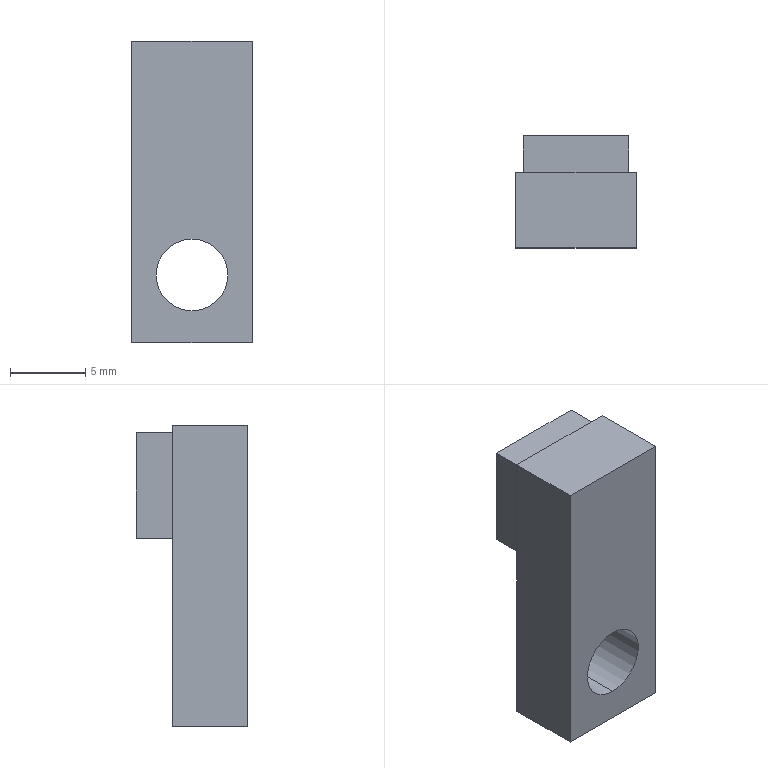Part | STEP file | 1_id1454_x_t | 1 solid | 13 faces | box 8 x 7.4 x 20 mm | volume 828.53 mm3 | plane 11 | cylinder 2 | commonest cylinder face diameters 4.763 x2
STEP:
#1=CARTESIAN_POINT('',(0.,0.,0.));
#2=DIRECTION('',(0.,0.,1.));
#3=DIRECTION('',(1.,0.,0.));
#4=AXIS2_PLACEMENT_3D('',#1,#2,#3);
#5=CARTESIAN_POINT('',(973.367,32.427,9.687));
#6=VERTEX_POINT('',#5);
#7=CARTESIAN_POINT('',(965.367,32.427,9.687));
#8=VERTEX_POINT('',#7);
#9=CARTESIAN_POINT('',(973.367,32.427,9.687));
#10=DIRECTION('',(-1.,0.,0.));
#11=VECTOR('',#10,1.);
#12=LINE('',#9,#11);
#13=CARTESIAN_POINT('',(969.367,32.427,9.687));
#14=DIRECTION('',(0.,1.,0.));
#15=DIRECTION('',(1.,0.,0.));
#16=AXIS2_PLACEMENT_3D('',#13,#14,#15);
#17=PLANE('',#16);
#18=CARTESIAN_POINT('',(4.,0.));
#19=DIRECTION('',(-1.,0.));
#20=VECTOR('',#19,1.);
#21=LINE('',#18,#20);
#22=(GEOMETRIC_REPRESENTATION_CONTEXT(2)PARAMETRIC_REPRESENTATION_CONTEXT()REPRESENTATION_CONTEXT('',''));
#23=DEFINITIONAL_REPRESENTATION('',(#21),#22);
#24=PCURVE('',#17,#23);
#25=CARTESIAN_POINT('',(969.367,29.927,9.687));
#26=DIRECTION('',(0.,0.,-1.));
#27=DIRECTION('',(0.,1.,0.));
#28=AXIS2_PLACEMENT_3D('',#25,#26,#27);
#29=PLANE('',#28);
#30=CARTESIAN_POINT('',(2.5,4.));
#31=DIRECTION('',(0.,-1.));
#32=VECTOR('',#31,1.);
#33=LINE('',#30,#32);
#34=(GEOMETRIC_REPRESENTATION_CONTEXT(2)PARAMETRIC_REPRESENTATION_CONTEXT()REPRESENTATION_CONTEXT('',''));
#35=DEFINITIONAL_REPRESENTATION('',(#33),#34);
#36=PCURVE('',#29,#35);
#37=SURFACE_CURVE('',#12,(#24,#36),.PCURVE_S1.);
#38=EDGE_CURVE('',#6,#8,#37,.T.);
#39=ORIENTED_EDGE('',*,*,#38,.T.);
#40=CARTESIAN_POINT('',(965.367,32.427,29.687));
#41=VERTEX_POINT('',#40);
#42=CARTESIAN_POINT('',(965.367,32.427,29.687));
#43=DIRECTION('',(0.,0.,-1.));
#44=VECTOR('',#43,1.);
#45=LINE('',#42,#44);
#46=CARTESIAN_POINT('',(-4.,-20.));
#47=DIRECTION('',(0.,1.));
#48=VECTOR('',#47,1.);
#49=LINE('',#46,#48);
#50=(GEOMETRIC_REPRESENTATION_CONTEXT(2)PARAMETRIC_REPRESENTATION_CONTEXT()REPRESENTATION_CONTEXT('',''));
#51=DEFINITIONAL_REPRESENTATION('',(#49),#50);
#52=PCURVE('',#17,#51);
#53=CARTESIAN_POINT('',(965.367,29.927,9.687));
#54=DIRECTION('',(-1.,0.,0.));
#55=DIRECTION('',(0.,-1.,0.));
#56=AXIS2_PLACEMENT_3D('',#53,#54,#55);
#57=PLANE('',#56);
#58=CARTESIAN_POINT('',(-2.5,20.));
#59=DIRECTION('',(0.,-1.));
#60=VECTOR('',#59,1.);
#61=LINE('',#58,#60);
#62=(GEOMETRIC_REPRESENTATION_CONTEXT(2)PARAMETRIC_REPRESENTATION_CONTEXT()REPRESENTATION_CONTEXT('',''));
#63=DEFINITIONAL_REPRESENTATION('',(#61),#62);
#64=PCURVE('',#57,#63);
#65=SURFACE_CURVE('',#45,(#52,#64),.PCURVE_S1.);
#66=EDGE_CURVE('',#41,#8,#65,.T.);
#67=ORIENTED_EDGE('',*,*,#66,.F.);
#68=CARTESIAN_POINT('',(973.367,32.427,29.687));
#69=VERTEX_POINT('',#68);
#70=CARTESIAN_POINT('',(965.367,32.427,29.687));
#71=DIRECTION('',(1.,0.,0.));
#72=VECTOR('',#71,1.);
#73=LINE('',#70,#72);
#74=CARTESIAN_POINT('',(-4.,-20.));
#75=DIRECTION('',(1.,0.));
#76=VECTOR('',#75,1.);
#77=LINE('',#74,#76);
#78=(GEOMETRIC_REPRESENTATION_CONTEXT(2)PARAMETRIC_REPRESENTATION_CONTEXT()REPRESENTATION_CONTEXT('',''));
#79=DEFINITIONAL_REPRESENTATION('',(#77),#78);
#80=PCURVE('',#17,#79);
#81=CARTESIAN_POINT('',(969.367,29.927,29.687));
#82=DIRECTION('',(0.,0.,1.));
#83=DIRECTION('',(1.,0.,0.));
#84=AXIS2_PLACEMENT_3D('',#81,#82,#83);
#85=PLANE('',#84);
#86=CARTESIAN_POINT('',(-4.,2.5));
#87=DIRECTION('',(1.,0.));
#88=VECTOR('',#87,1.);
#89=LINE('',#86,#88);
#90=(GEOMETRIC_REPRESENTATION_CONTEXT(2)PARAMETRIC_REPRESENTATION_CONTEXT()REPRESENTATION_CONTEXT('',''));
#91=DEFINITIONAL_REPRESENTATION('',(#89),#90);
#92=PCURVE('',#85,#91);
#93=SURFACE_CURVE('',#73,(#80,#92),.PCURVE_S1.);
#94=EDGE_CURVE('',#41,#69,#93,.T.);
#95=ORIENTED_EDGE('',*,*,#94,.T.);
#96=CARTESIAN_POINT('',(973.367,32.427,29.687));
#97=DIRECTION('',(0.,0.,-1.));
#98=VECTOR('',#97,1.);
#99=LINE('',#96,#98);
#100=CARTESIAN_POINT('',(4.,-20.));
#101=DIRECTION('',(0.,1.));
#102=VECTOR('',#101,1.);
#103=LINE('',#100,#102);
#104=(GEOMETRIC_REPRESENTATION_CONTEXT(2)PARAMETRIC_REPRESENTATION_CONTEXT()REPRESENTATION_CONTEXT('',''));
#105=DEFINITIONAL_REPRESENTATION('',(#103),#104);
#106=PCURVE('',#17,#105);
#107=CARTESIAN_POINT('',(973.367,29.927,9.687));
#108=DIRECTION('',(1.,0.,0.));
#109=DIRECTION('',(0.,-1.,0.));
#110=AXIS2_PLACEMENT_3D('',#107,#108,#109);
#111=PLANE('',#110);
#112=CARTESIAN_POINT('',(-2.5,-20.));
#113=DIRECTION('',(0.,1.));
#114=VECTOR('',#113,1.);
#115=LINE('',#112,#114);
#116=(GEOMETRIC_REPRESENTATION_CONTEXT(2)PARAMETRIC_REPRESENTATION_CONTEXT()REPRESENTATION_CONTEXT('',''));
#117=DEFINITIONAL_REPRESENTATION('',(#115),#116);
#118=PCURVE('',#111,#117);
#119=SURFACE_CURVE('',#99,(#106,#118),.PCURVE_S1.);
#120=EDGE_CURVE('',#69,#6,#119,.T.);
#121=ORIENTED_EDGE('',*,*,#120,.T.);
#122=EDGE_LOOP('',(#39,#67,#95,#121));
#123=FACE_BOUND('',#122,.T.);
#124=CARTESIAN_POINT('',(969.367,32.427,16.569));
#125=VERTEX_POINT('',#124);
#126=CARTESIAN_POINT('',(969.367,32.427,11.806));
#127=VERTEX_POINT('',#126);
#128=CARTESIAN_POINT('',(969.367,32.427,14.187));
#129=DIRECTION('',(0.,-1.,0.));
#130=DIRECTION('',(0.,0.,1.));
#131=AXIS2_PLACEMENT_3D('',#128,#129,#130);
#132=CIRCLE('',#131,2.381);
#133=CARTESIAN_POINT('',(0.,-6.881));
#134=CARTESIAN_POINT('',(-4.124,-6.881));
#135=CARTESIAN_POINT('',(-2.062,-3.309));
#136=CARTESIAN_POINT('',(0.,0.2625));
#137=CARTESIAN_POINT('',(2.062,-3.309));
#138=CARTESIAN_POINT('',(4.124,-6.881));
#139=CARTESIAN_POINT('',(0.,-6.881));
#140=(BOUNDED_CURVE()B_SPLINE_CURVE(2,(#133,#134,#135,#136,#137,#138,#139),.UNSPECIFIED.,.T.,.F.)B_SPLINE_CURVE_WITH_KNOTS((1,2,2,2,2,1),(-2.094,0.,2.094,4.189,6.283,8.378),.UNSPECIFIED.)CURVE()GEOMETRIC_REPRESENTATION_ITEM()RATIONAL_B_SPLINE_CURVE((1.,0.5,1.,0.5,1.,0.5,1.))REPRESENTATION_ITEM(''));
#141=(GEOMETRIC_REPRESENTATION_CONTEXT(2)PARAMETRIC_REPRESENTATION_CONTEXT()REPRESENTATION_CONTEXT('',''));
#142=DEFINITIONAL_REPRESENTATION('',(#140),#141);
#143=PCURVE('',#17,#142);
#144=CARTESIAN_POINT('',(969.367,32.427,14.187));
#145=DIRECTION('',(0.,1.,0.));
#146=DIRECTION('',(0.,0.,1.));
#147=AXIS2_PLACEMENT_3D('',#144,#145,#146);
#148=CYLINDRICAL_SURFACE('',#147,2.381);
#149=CARTESIAN_POINT('',(6.283,0.));
#150=DIRECTION('',(-1.,0.));
#151=VECTOR('',#150,1.);
#152=LINE('',#149,#151);
#153=(GEOMETRIC_REPRESENTATION_CONTEXT(2)PARAMETRIC_REPRESENTATION_CONTEXT()REPRESENTATION_CONTEXT('',''));
#154=DEFINITIONAL_REPRESENTATION('',(#152),#153);
#155=PCURVE('',#148,#154);
#156=SURFACE_CURVE('',#132,(#143,#155),.PCURVE_S1.);
#157=EDGE_CURVE('',#125,#127,#156,.T.);
#158=ORIENTED_EDGE('',*,*,#157,.T.);
#159=CARTESIAN_POINT('',(969.367,32.427,14.187));
#160=DIRECTION('',(0.,-1.,0.));
#161=DIRECTION('',(0.,0.,-1.));
#162=AXIS2_PLACEMENT_3D('',#159,#160,#161);
#163=CIRCLE('',#162,2.381);
#164=CARTESIAN_POINT('',(0.,-2.119));
#165=CARTESIAN_POINT('',(4.124,-2.119));
#166=CARTESIAN_POINT('',(2.062,-5.691));
#167=CARTESIAN_POINT('',(0.,-9.262));
#168=CARTESIAN_POINT('',(-2.062,-5.691));
#169=CARTESIAN_POINT('',(-4.124,-2.119));
#170=CARTESIAN_POINT('',(0.,-2.119));
#171=(BOUNDED_CURVE()B_SPLINE_CURVE(2,(#164,#165,#166,#167,#168,#169,#170),.UNSPECIFIED.,.T.,.F.)B_SPLINE_CURVE_WITH_KNOTS((1,2,2,2,2,1),(-2.094,0.,2.094,4.189,6.283,8.378),.UNSPECIFIED.)CURVE()GEOMETRIC_REPRESENTATION_ITEM()RATIONAL_B_SPLINE_CURVE((1.,0.5,1.,0.5,1.,0.5,1.))REPRESENTATION_ITEM(''));
#172=(GEOMETRIC_REPRESENTATION_CONTEXT(2)PARAMETRIC_REPRESENTATION_CONTEXT()REPRESENTATION_CONTEXT('',''));
#173=DEFINITIONAL_REPRESENTATION('',(#171),#172);
#174=PCURVE('',#17,#173);
#175=CARTESIAN_POINT('',(969.367,32.427,14.187));
#176=DIRECTION('',(0.,1.,0.));
#177=DIRECTION('',(0.,0.,1.));
#178=AXIS2_PLACEMENT_3D('',#175,#176,#177);
#179=CYLINDRICAL_SURFACE('',#178,2.381);
#180=CARTESIAN_POINT('',(3.142,0.));
#181=DIRECTION('',(-1.,0.));
#182=VECTOR('',#181,1.);
#183=LINE('',#180,#182);
#184=(GEOMETRIC_REPRESENTATION_CONTEXT(2)PARAMETRIC_REPRESENTATION_CONTEXT()REPRESENTATION_CONTEXT('',''));
#185=DEFINITIONAL_REPRESENTATION('',(#183),#184);
#186=PCURVE('',#179,#185);
#187=SURFACE_CURVE('',#163,(#174,#186),.PCURVE_S1.);
#188=EDGE_CURVE('',#127,#125,#187,.T.);
#189=ORIENTED_EDGE('',*,*,#188,.T.);
#190=EDGE_LOOP('',(#158,#189));
#191=FACE_BOUND('',#190,.T.);
#192=CARTESIAN_POINT('',(972.867,32.427,22.187));
#193=VERTEX_POINT('',#192);
#194=CARTESIAN_POINT('',(965.867,32.427,22.187));
#195=VERTEX_POINT('',#194);
#196=CARTESIAN_POINT('',(972.867,32.427,22.187));
#197=DIRECTION('',(-1.,0.,0.));
#198=VECTOR('',#197,1.);
#199=LINE('',#196,#198);
#200=CARTESIAN_POINT('',(3.5,-12.5));
#201=DIRECTION('',(-1.,0.));
#202=VECTOR('',#201,1.);
#203=LINE('',#200,#202);
#204=(GEOMETRIC_REPRESENTATION_CONTEXT(2)PARAMETRIC_REPRESENTATION_CONTEXT()REPRESENTATION_CONTEXT('',''));
#205=DEFINITIONAL_REPRESENTATION('',(#203),#204);
#206=PCURVE('',#17,#205);
#207=CARTESIAN_POINT('',(972.867,32.427,22.187));
#208=DIRECTION('',(0.,0.,-1.));
#209=DIRECTION('',(0.,1.,0.));
#210=AXIS2_PLACEMENT_3D('',#207,#208,#209);
#211=PLANE('',#210);
#212=CARTESIAN_POINT('',(0.,0.));
#213=DIRECTION('',(0.,-1.));
#214=VECTOR('',#213,1.);
#215=LINE('',#212,#214);
#216=(GEOMETRIC_REPRESENTATION_CONTEXT(2)PARAMETRIC_REPRESENTATION_CONTEXT()REPRESENTATION_CONTEXT('',''));
#217=DEFINITIONAL_REPRESENTATION('',(#215),#216);
#218=PCURVE('',#211,#217);
#219=SURFACE_CURVE('',#199,(#206,#218),.PCURVE_S1.);
#220=EDGE_CURVE('',#193,#195,#219,.T.);
#221=ORIENTED_EDGE('',*,*,#220,.F.);
#222=CARTESIAN_POINT('',(972.867,32.427,29.187));
#223=VERTEX_POINT('',#222);
#224=CARTESIAN_POINT('',(972.867,32.427,29.187));
#225=DIRECTION('',(0.,0.,-1.));
#226=VECTOR('',#225,1.);
#227=LINE('',#224,#226);
#228=CARTESIAN_POINT('',(3.5,-19.5));
#229=DIRECTION('',(0.,1.));
#230=VECTOR('',#229,1.);
#231=LINE('',#228,#230);
#232=(GEOMETRIC_REPRESENTATION_CONTEXT(2)PARAMETRIC_REPRESENTATION_CONTEXT()REPRESENTATION_CONTEXT('',''));
#233=DEFINITIONAL_REPRESENTATION('',(#231),#232);
#234=PCURVE('',#17,#233);
#235=CARTESIAN_POINT('',(972.867,32.427,29.187));
#236=DIRECTION('',(1.,0.,0.));
#237=DIRECTION('',(0.,-1.,0.));
#238=AXIS2_PLACEMENT_3D('',#235,#236,#237);
#239=PLANE('',#238);
#240=CARTESIAN_POINT('',(0.,0.));
#241=DIRECTION('',(0.,1.));
#242=VECTOR('',#241,1.);
#243=LINE('',#240,#242);
#244=(GEOMETRIC_REPRESENTATION_CONTEXT(2)PARAMETRIC_REPRESENTATION_CONTEXT()REPRESENTATION_CONTEXT('',''));
#245=DEFINITIONAL_REPRESENTATION('',(#243),#244);
#246=PCURVE('',#239,#245);
#247=SURFACE_CURVE('',#227,(#234,#246),.PCURVE_S1.);
#248=EDGE_CURVE('',#223,#193,#247,.T.);
#249=ORIENTED_EDGE('',*,*,#248,.F.);
#250=CARTESIAN_POINT('',(965.867,32.427,29.187));
#251=VERTEX_POINT('',#250);
#252=CARTESIAN_POINT('',(972.867,32.427,29.187));
#253=DIRECTION('',(-1.,0.,0.));
#254=VECTOR('',#253,1.);
#255=LINE('',#252,#254);
#256=CARTESIAN_POINT('',(3.5,-19.5));
#257=DIRECTION('',(-1.,0.));
#258=VECTOR('',#257,1.);
#259=LINE('',#256,#258);
#260=(GEOMETRIC_REPRESENTATION_CONTEXT(2)PARAMETRIC_REPRESENTATION_CONTEXT()REPRESENTATION_CONTEXT('',''));
#261=DEFINITIONAL_REPRESENTATION('',(#259),#260);
#262=PCURVE('',#17,#261);
#263=CARTESIAN_POINT('',(965.867,32.427,29.187));
#264=DIRECTION('',(0.,0.,1.));
#265=DIRECTION('',(1.,0.,0.));
#266=AXIS2_PLACEMENT_3D('',#263,#264,#265);
#267=PLANE('',#266);
#268=CARTESIAN_POINT('',(7.,0.));
#269=DIRECTION('',(-1.,0.));
#270=VECTOR('',#269,1.);
#271=LINE('',#268,#270);
#272=(GEOMETRIC_REPRESENTATION_CONTEXT(2)PARAMETRIC_REPRESENTATION_CONTEXT()REPRESENTATION_CONTEXT('',''));
#273=DEFINITIONAL_REPRESENTATION('',(#271),#272);
#274=PCURVE('',#267,#273);
#275=SURFACE_CURVE('',#255,(#262,#274),.PCURVE_S1.);
#276=EDGE_CURVE('',#223,#251,#275,.T.);
#277=ORIENTED_EDGE('',*,*,#276,.T.);
#278=CARTESIAN_POINT('',(965.867,32.427,29.187));
#279=DIRECTION('',(0.,0.,-1.));
#280=VECTOR('',#279,1.);
#281=LINE('',#278,#280);
#282=CARTESIAN_POINT('',(-3.5,-19.5));
#283=DIRECTION('',(0.,1.));
#284=VECTOR('',#283,1.);
#285=LINE('',#282,#284);
#286=(GEOMETRIC_REPRESENTATION_CONTEXT(2)PARAMETRIC_REPRESENTATION_CONTEXT()REPRESENTATION_CONTEXT('',''));
#287=DEFINITIONAL_REPRESENTATION('',(#285),#286);
#288=PCURVE('',#17,#287);
#289=CARTESIAN_POINT('',(965.867,32.427,22.187));
#290=DIRECTION('',(-1.,0.,0.));
#291=DIRECTION('',(0.,-1.,0.));
#292=AXIS2_PLACEMENT_3D('',#289,#290,#291);
#293=PLANE('',#292);
#294=CARTESIAN_POINT('',(0.,7.));
#295=DIRECTION('',(0.,-1.));
#296=VECTOR('',#295,1.);
#297=LINE('',#294,#296);
#298=(GEOMETRIC_REPRESENTATION_CONTEXT(2)PARAMETRIC_REPRESENTATION_CONTEXT()REPRESENTATION_CONTEXT('',''));
#299=DEFINITIONAL_REPRESENTATION('',(#297),#298);
#300=PCURVE('',#293,#299);
#301=SURFACE_CURVE('',#281,(#288,#300),.PCURVE_S1.);
#302=EDGE_CURVE('',#251,#195,#301,.T.);
#303=ORIENTED_EDGE('',*,*,#302,.T.);
#304=EDGE_LOOP('',(#221,#249,#277,#303));
#305=FACE_BOUND('',#304,.T.);
#306=ADVANCED_FACE('',(#123,#191,#305),#17,.T.);
#307=CARTESIAN_POINT('',(973.367,27.427,9.687));
#308=VERTEX_POINT('',#307);
#309=CARTESIAN_POINT('',(973.367,27.427,9.687));
#310=DIRECTION('',(0.,1.,0.));
#311=VECTOR('',#310,1.);
#312=LINE('',#309,#311);
#313=CARTESIAN_POINT('',(2.5,0.));
#314=DIRECTION('',(-1.,0.));
#315=VECTOR('',#314,1.);
#316=LINE('',#313,#315);
#317=(GEOMETRIC_REPRESENTATION_CONTEXT(2)PARAMETRIC_REPRESENTATION_CONTEXT()REPRESENTATION_CONTEXT('',''));
#318=DEFINITIONAL_REPRESENTATION('',(#316),#317);
#319=PCURVE('',#111,#318);
#320=CARTESIAN_POINT('',(-2.5,4.));
#321=DIRECTION('',(1.,0.));
#322=VECTOR('',#321,1.);
#323=LINE('',#320,#322);
#324=(GEOMETRIC_REPRESENTATION_CONTEXT(2)PARAMETRIC_REPRESENTATION_CONTEXT()REPRESENTATION_CONTEXT('',''));
#325=DEFINITIONAL_REPRESENTATION('',(#323),#324);
#326=PCURVE('',#29,#325);
#327=SURFACE_CURVE('',#312,(#319,#326),.PCURVE_S1.);
#328=EDGE_CURVE('',#308,#6,#327,.T.);
#329=ORIENTED_EDGE('',*,*,#328,.T.);
#330=ORIENTED_EDGE('',*,*,#120,.F.);
#331=CARTESIAN_POINT('',(973.367,27.427,29.687));
#332=VERTEX_POINT('',#331);
#333=CARTESIAN_POINT('',(973.367,32.427,29.687));
#334=DIRECTION('',(0.,-1.,0.));
#335=VECTOR('',#334,1.);
#336=LINE('',#333,#335);
#337=CARTESIAN_POINT('',(-2.5,-20.));
#338=DIRECTION('',(1.,0.));
#339=VECTOR('',#338,1.);
#340=LINE('',#337,#339);
#341=(GEOMETRIC_REPRESENTATION_CONTEXT(2)PARAMETRIC_REPRESENTATION_CONTEXT()REPRESENTATION_CONTEXT('',''));
#342=DEFINITIONAL_REPRESENTATION('',(#340),#341);
#343=PCURVE('',#111,#342);
#344=CARTESIAN_POINT('',(4.,2.5));
#345=DIRECTION('',(0.,-1.));
#346=VECTOR('',#345,1.);
#347=LINE('',#344,#346);
#348=(GEOMETRIC_REPRESENTATION_CONTEXT(2)PARAMETRIC_REPRESENTATION_CONTEXT()REPRESENTATION_CONTEXT('',''));
#349=DEFINITIONAL_REPRESENTATION('',(#347),#348);
#350=PCURVE('',#85,#349);
#351=SURFACE_CURVE('',#336,(#343,#350),.PCURVE_S1.);
#352=EDGE_CURVE('',#69,#332,#351,.T.);
#353=ORIENTED_EDGE('',*,*,#352,.T.);
#354=CARTESIAN_POINT('',(973.367,27.427,29.687));
#355=DIRECTION('',(0.,0.,-1.));
#356=VECTOR('',#355,1.);
#357=LINE('',#354,#356);
#358=CARTESIAN_POINT('',(2.5,-20.));
#359=DIRECTION('',(0.,1.));
#360=VECTOR('',#359,1.);
#361=LINE('',#358,#360);
#362=(GEOMETRIC_REPRESENTATION_CONTEXT(2)PARAMETRIC_REPRESENTATION_CONTEXT()REPRESENTATION_CONTEXT('',''));
#363=DEFINITIONAL_REPRESENTATION('',(#361),#362);
#364=PCURVE('',#111,#363);
#365=CARTESIAN_POINT('',(969.367,27.427,9.687));
#366=DIRECTION('',(0.,-1.,0.));
#367=DIRECTION('',(0.,0.,1.));
#368=AXIS2_PLACEMENT_3D('',#365,#366,#367);
#369=PLANE('',#368);
#370=CARTESIAN_POINT('',(20.,-4.));
#371=DIRECTION('',(-1.,0.));
#372=VECTOR('',#371,1.);
#373=LINE('',#370,#372);
#374=(GEOMETRIC_REPRESENTATION_CONTEXT(2)PARAMETRIC_REPRESENTATION_CONTEXT()REPRESENTATION_CONTEXT('',''));
#375=DEFINITIONAL_REPRESENTATION('',(#373),#374);
#376=PCURVE('',#369,#375);
#377=SURFACE_CURVE('',#357,(#364,#376),.PCURVE_S1.);
#378=EDGE_CURVE('',#332,#308,#377,.T.);
#379=ORIENTED_EDGE('',*,*,#378,.T.);
#380=EDGE_LOOP('',(#329,#330,#353,#379));
#381=FACE_BOUND('',#380,.T.);
#382=ADVANCED_FACE('',(#381),#111,.T.);
#383=ORIENTED_EDGE('',*,*,#378,.F.);
#384=CARTESIAN_POINT('',(965.367,27.427,29.687));
#385=VERTEX_POINT('',#384);
#386=CARTESIAN_POINT('',(973.367,27.427,29.687));
#387=DIRECTION('',(-1.,0.,0.));
#388=VECTOR('',#387,1.);
#389=LINE('',#386,#388);
#390=CARTESIAN_POINT('',(20.,-4.));
#391=DIRECTION('',(0.,1.));
#392=VECTOR('',#391,1.);
#393=LINE('',#390,#392);
#394=(GEOMETRIC_REPRESENTATION_CONTEXT(2)PARAMETRIC_REPRESENTATION_CONTEXT()REPRESENTATION_CONTEXT('',''));
#395=DEFINITIONAL_REPRESENTATION('',(#393),#394);
#396=PCURVE('',#369,#395);
#397=CARTESIAN_POINT('',(4.,-2.5));
#398=DIRECTION('',(-1.,0.));
#399=VECTOR('',#398,1.);
#400=LINE('',#397,#399);
#401=(GEOMETRIC_REPRESENTATION_CONTEXT(2)PARAMETRIC_REPRESENTATION_CONTEXT()REPRESENTATION_CONTEXT('',''));
#402=DEFINITIONAL_REPRESENTATION('',(#400),#401);
#403=PCURVE('',#85,#402);
#404=SURFACE_CURVE('',#389,(#396,#403),.PCURVE_S1.);
#405=EDGE_CURVE('',#332,#385,#404,.T.);
#406=ORIENTED_EDGE('',*,*,#405,.T.);
#407=CARTESIAN_POINT('',(965.367,27.427,9.687));
#408=VERTEX_POINT('',#407);
#409=CARTESIAN_POINT('',(965.367,27.427,29.687));
#410=DIRECTION('',(0.,0.,-1.));
#411=VECTOR('',#410,1.);
#412=LINE('',#409,#411);
#413=CARTESIAN_POINT('',(20.,4.));
#414=DIRECTION('',(-1.,0.));
#415=VECTOR('',#414,1.);
#416=LINE('',#413,#415);
#417=(GEOMETRIC_REPRESENTATION_CONTEXT(2)PARAMETRIC_REPRESENTATION_CONTEXT()REPRESENTATION_CONTEXT('',''));
#418=DEFINITIONAL_REPRESENTATION('',(#416),#417);
#419=PCURVE('',#369,#418);
#420=CARTESIAN_POINT('',(2.5,20.));
#421=DIRECTION('',(0.,-1.));
#422=VECTOR('',#421,1.);
#423=LINE('',#420,#422);
#424=(GEOMETRIC_REPRESENTATION_CONTEXT(2)PARAMETRIC_REPRESENTATION_CONTEXT()REPRESENTATION_CONTEXT('',''));
#425=DEFINITIONAL_REPRESENTATION('',(#423),#424);
#426=PCURVE('',#57,#425);
#427=SURFACE_CURVE('',#412,(#419,#426),.PCURVE_S1.);
#428=EDGE_CURVE('',#385,#408,#427,.T.);
#429=ORIENTED_EDGE('',*,*,#428,.T.);
#430=CARTESIAN_POINT('',(965.367,27.427,9.687));
#431=DIRECTION('',(1.,0.,0.));
#432=VECTOR('',#431,1.);
#433=LINE('',#430,#432);
#434=CARTESIAN_POINT('',(0.,4.));
#435=DIRECTION('',(0.,-1.));
#436=VECTOR('',#435,1.);
#437=LINE('',#434,#436);
#438=(GEOMETRIC_REPRESENTATION_CONTEXT(2)PARAMETRIC_REPRESENTATION_CONTEXT()REPRESENTATION_CONTEXT('',''));
#439=DEFINITIONAL_REPRESENTATION('',(#437),#438);
#440=PCURVE('',#369,#439);
#441=CARTESIAN_POINT('',(-2.5,-4.));
#442=DIRECTION('',(0.,1.));
#443=VECTOR('',#442,1.);
#444=LINE('',#441,#443);
#445=(GEOMETRIC_REPRESENTATION_CONTEXT(2)PARAMETRIC_REPRESENTATION_CONTEXT()REPRESENTATION_CONTEXT('',''));
#446=DEFINITIONAL_REPRESENTATION('',(#444),#445);
#447=PCURVE('',#29,#446);
#448=SURFACE_CURVE('',#433,(#440,#447),.PCURVE_S1.);
#449=EDGE_CURVE('',#408,#308,#448,.T.);
#450=ORIENTED_EDGE('',*,*,#449,.T.);
#451=EDGE_LOOP('',(#383,#406,#429,#450));
#452=FACE_BOUND('',#451,.T.);
#453=CARTESIAN_POINT('',(969.367,27.427,16.569));
#454=VERTEX_POINT('',#453);
#455=CARTESIAN_POINT('',(969.367,27.427,11.806));
#456=VERTEX_POINT('',#455);
#457=CARTESIAN_POINT('',(969.367,27.427,14.187));
#458=DIRECTION('',(0.,1.,0.));
#459=DIRECTION('',(0.,0.,1.));
#460=AXIS2_PLACEMENT_3D('',#457,#458,#459);
#461=CIRCLE('',#460,2.381);
#462=CARTESIAN_POINT('',(6.881,0.));
#463=CARTESIAN_POINT('',(6.881,-4.124));
#464=CARTESIAN_POINT('',(3.309,-2.062));
#465=CARTESIAN_POINT('',(-0.2625,0.));
#466=CARTESIAN_POINT('',(3.309,2.062));
#467=CARTESIAN_POINT('',(6.881,4.124));
#468=CARTESIAN_POINT('',(6.881,0.));
#469=(BOUNDED_CURVE()B_SPLINE_CURVE(2,(#462,#463,#464,#465,#466,#467,#468),.UNSPECIFIED.,.T.,.F.)B_SPLINE_CURVE_WITH_KNOTS((1,2,2,2,2,1),(-2.094,0.,2.094,4.189,6.283,8.378),.UNSPECIFIED.)CURVE()GEOMETRIC_REPRESENTATION_ITEM()RATIONAL_B_SPLINE_CURVE((1.,0.5,1.,0.5,1.,0.5,1.))REPRESENTATION_ITEM(''));
#470=(GEOMETRIC_REPRESENTATION_CONTEXT(2)PARAMETRIC_REPRESENTATION_CONTEXT()REPRESENTATION_CONTEXT('',''));
#471=DEFINITIONAL_REPRESENTATION('',(#469),#470);
#472=PCURVE('',#369,#471);
#473=CARTESIAN_POINT('',(0.,-5.));
#474=DIRECTION('',(1.,0.));
#475=VECTOR('',#474,1.);
#476=LINE('',#473,#475);
#477=(GEOMETRIC_REPRESENTATION_CONTEXT(2)PARAMETRIC_REPRESENTATION_CONTEXT()REPRESENTATION_CONTEXT('',''));
#478=DEFINITIONAL_REPRESENTATION('',(#476),#477);
#479=PCURVE('',#179,#478);
#480=SURFACE_CURVE('',#461,(#472,#479),.PCURVE_S1.);
#481=EDGE_CURVE('',#454,#456,#480,.T.);
#482=ORIENTED_EDGE('',*,*,#481,.T.);
#483=CARTESIAN_POINT('',(969.367,27.427,14.187));
#484=DIRECTION('',(0.,1.,0.));
#485=DIRECTION('',(0.,0.,-1.));
#486=AXIS2_PLACEMENT_3D('',#483,#484,#485);
#487=CIRCLE('',#486,2.381);
#488=CARTESIAN_POINT('',(2.119,0.));
#489=CARTESIAN_POINT('',(2.119,4.124));
#490=CARTESIAN_POINT('',(5.691,2.062));
#491=CARTESIAN_POINT('',(9.262,0.));
#492=CARTESIAN_POINT('',(5.691,-2.062));
#493=CARTESIAN_POINT('',(2.119,-4.124));
#494=CARTESIAN_POINT('',(2.119,0.));
#495=(BOUNDED_CURVE()B_SPLINE_CURVE(2,(#488,#489,#490,#491,#492,#493,#494),.UNSPECIFIED.,.T.,.F.)B_SPLINE_CURVE_WITH_KNOTS((1,2,2,2,2,1),(-2.094,0.,2.094,4.189,6.283,8.378),.UNSPECIFIED.)CURVE()GEOMETRIC_REPRESENTATION_ITEM()RATIONAL_B_SPLINE_CURVE((1.,0.5,1.,0.5,1.,0.5,1.))REPRESENTATION_ITEM(''));
#496=(GEOMETRIC_REPRESENTATION_CONTEXT(2)PARAMETRIC_REPRESENTATION_CONTEXT()REPRESENTATION_CONTEXT('',''));
#497=DEFINITIONAL_REPRESENTATION('',(#495),#496);
#498=PCURVE('',#369,#497);
#499=CARTESIAN_POINT('',(3.142,-5.));
#500=DIRECTION('',(1.,0.));
#501=VECTOR('',#500,1.);
#502=LINE('',#499,#501);
#503=(GEOMETRIC_REPRESENTATION_CONTEXT(2)PARAMETRIC_REPRESENTATION_CONTEXT()REPRESENTATION_CONTEXT('',''));
#504=DEFINITIONAL_REPRESENTATION('',(#502),#503);
#505=PCURVE('',#148,#504);
#506=SURFACE_CURVE('',#487,(#498,#505),.PCURVE_S1.);
#507=EDGE_CURVE('',#456,#454,#506,.T.);
#508=ORIENTED_EDGE('',*,*,#507,.T.);
#509=EDGE_LOOP('',(#482,#508));
#510=FACE_BOUND('',#509,.T.);
#511=ADVANCED_FACE('',(#452,#510),#369,.T.);
#512=CARTESIAN_POINT('',(965.367,32.427,9.687));
#513=DIRECTION('',(0.,-1.,0.));
#514=VECTOR('',#513,1.);
#515=LINE('',#512,#514);
#516=CARTESIAN_POINT('',(2.5,-4.));
#517=DIRECTION('',(-1.,0.));
#518=VECTOR('',#517,1.);
#519=LINE('',#516,#518);
#520=(GEOMETRIC_REPRESENTATION_CONTEXT(2)PARAMETRIC_REPRESENTATION_CONTEXT()REPRESENTATION_CONTEXT('',''));
#521=DEFINITIONAL_REPRESENTATION('',(#519),#520);
#522=PCURVE('',#29,#521);
#523=CARTESIAN_POINT('',(-2.5,0.));
#524=DIRECTION('',(1.,0.));
#525=VECTOR('',#524,1.);
#526=LINE('',#523,#525);
#527=(GEOMETRIC_REPRESENTATION_CONTEXT(2)PARAMETRIC_REPRESENTATION_CONTEXT()REPRESENTATION_CONTEXT('',''));
#528=DEFINITIONAL_REPRESENTATION('',(#526),#527);
#529=PCURVE('',#57,#528);
#530=SURFACE_CURVE('',#515,(#522,#529),.PCURVE_S1.);
#531=EDGE_CURVE('',#8,#408,#530,.T.);
#532=ORIENTED_EDGE('',*,*,#531,.F.);
#533=ORIENTED_EDGE('',*,*,#38,.F.);
#534=ORIENTED_EDGE('',*,*,#328,.F.);
#535=ORIENTED_EDGE('',*,*,#449,.F.);
#536=EDGE_LOOP('',(#532,#533,#534,#535));
#537=FACE_BOUND('',#536,.T.);
#538=ADVANCED_FACE('',(#537),#29,.T.);
#539=ORIENTED_EDGE('',*,*,#531,.T.);
#540=ORIENTED_EDGE('',*,*,#428,.F.);
#541=CARTESIAN_POINT('',(965.367,27.427,29.687));
#542=DIRECTION('',(0.,1.,0.));
#543=VECTOR('',#542,1.);
#544=LINE('',#541,#543);
#545=CARTESIAN_POINT('',(2.5,20.));
#546=DIRECTION('',(-1.,0.));
#547=VECTOR('',#546,1.);
#548=LINE('',#545,#547);
#549=(GEOMETRIC_REPRESENTATION_CONTEXT(2)PARAMETRIC_REPRESENTATION_CONTEXT()REPRESENTATION_CONTEXT('',''));
#550=DEFINITIONAL_REPRESENTATION('',(#548),#549);
#551=PCURVE('',#57,#550);
#552=CARTESIAN_POINT('',(-4.,-2.5));
#553=DIRECTION('',(0.,1.));
#554=VECTOR('',#553,1.);
#555=LINE('',#552,#554);
#556=(GEOMETRIC_REPRESENTATION_CONTEXT(2)PARAMETRIC_REPRESENTATION_CONTEXT()REPRESENTATION_CONTEXT('',''));
#557=DEFINITIONAL_REPRESENTATION('',(#555),#556);
#558=PCURVE('',#85,#557);
#559=SURFACE_CURVE('',#544,(#551,#558),.PCURVE_S1.);
#560=EDGE_CURVE('',#385,#41,#559,.T.);
#561=ORIENTED_EDGE('',*,*,#560,.T.);
#562=ORIENTED_EDGE('',*,*,#66,.T.);
#563=EDGE_LOOP('',(#539,#540,#561,#562));
#564=FACE_BOUND('',#563,.T.);
#565=ADVANCED_FACE('',(#564),#57,.T.);
#566=ORIENTED_EDGE('',*,*,#94,.F.);
#567=ORIENTED_EDGE('',*,*,#560,.F.);
#568=ORIENTED_EDGE('',*,*,#405,.F.);
#569=ORIENTED_EDGE('',*,*,#352,.F.);
#570=EDGE_LOOP('',(#566,#567,#568,#569));
#571=FACE_BOUND('',#570,.T.);
#572=ADVANCED_FACE('',(#571),#85,.T.);
#573=ORIENTED_EDGE('',*,*,#157,.T.);
#574=CARTESIAN_POINT('',(969.367,27.427,11.806));
#575=DIRECTION('',(0.,1.,0.));
#576=VECTOR('',#575,1.);
#577=LINE('',#574,#576);
#578=CARTESIAN_POINT('',(3.142,-5.));
#579=DIRECTION('',(0.,1.));
#580=VECTOR('',#579,1.);
#581=LINE('',#578,#580);
#582=(GEOMETRIC_REPRESENTATION_CONTEXT(2)PARAMETRIC_REPRESENTATION_CONTEXT()REPRESENTATION_CONTEXT('',''));
#583=DEFINITIONAL_REPRESENTATION('',(#581),#582);
#584=PCURVE('',#148,#583);
#585=CARTESIAN_POINT('',(3.142,-5.));
#586=DIRECTION('',(0.,1.));
#587=VECTOR('',#586,1.);
#588=LINE('',#585,#587);
#589=(GEOMETRIC_REPRESENTATION_CONTEXT(2)PARAMETRIC_REPRESENTATION_CONTEXT()REPRESENTATION_CONTEXT('',''));
#590=DEFINITIONAL_REPRESENTATION('',(#588),#589);
#591=PCURVE('',#179,#590);
#592=SURFACE_CURVE('',#577,(#584,#591),.PCURVE_S1.);
#593=EDGE_CURVE('',#456,#127,#592,.T.);
#594=ORIENTED_EDGE('',*,*,#593,.F.);
#595=ORIENTED_EDGE('',*,*,#507,.T.);
#596=CARTESIAN_POINT('',(969.367,27.427,16.569));
#597=DIRECTION('',(0.,-1.,0.));
#598=VECTOR('',#597,1.);
#599=LINE('',#596,#598);
#600=CARTESIAN_POINT('',(6.283,-5.));
#601=DIRECTION('',(0.,-1.));
#602=VECTOR('',#601,1.);
#603=LINE('',#600,#602);
#604=(GEOMETRIC_REPRESENTATION_CONTEXT(2)PARAMETRIC_REPRESENTATION_CONTEXT()REPRESENTATION_CONTEXT('',''));
#605=DEFINITIONAL_REPRESENTATION('',(#603),#604);
#606=PCURVE('',#148,#605);
#607=CARTESIAN_POINT('',(0.,-5.));
#608=DIRECTION('',(0.,-1.));
#609=VECTOR('',#608,1.);
#610=LINE('',#607,#609);
#611=(GEOMETRIC_REPRESENTATION_CONTEXT(2)PARAMETRIC_REPRESENTATION_CONTEXT()REPRESENTATION_CONTEXT('',''));
#612=DEFINITIONAL_REPRESENTATION('',(#610),#611);
#613=PCURVE('',#179,#612);
#614=SURFACE_CURVE('',#599,(#606,#613),.PCURVE_S1.);
#615=EDGE_CURVE('',#125,#454,#614,.T.);
#616=ORIENTED_EDGE('',*,*,#615,.F.);
#617=EDGE_LOOP('',(#573,#594,#595,#616));
#618=FACE_BOUND('',#617,.F.);
#619=ADVANCED_FACE('',(#618),#148,.F.);
#620=ORIENTED_EDGE('',*,*,#188,.T.);
#621=ORIENTED_EDGE('',*,*,#615,.T.);
#622=ORIENTED_EDGE('',*,*,#481,.T.);
#623=ORIENTED_EDGE('',*,*,#593,.T.);
#624=EDGE_LOOP('',(#620,#621,#622,#623));
#625=FACE_BOUND('',#624,.F.);
#626=ADVANCED_FACE('',(#625),#179,.F.);
#627=CARTESIAN_POINT('',(965.867,34.827,29.187));
#628=VERTEX_POINT('',#627);
#629=CARTESIAN_POINT('',(965.867,34.827,29.187));
#630=DIRECTION('',(0.,-1.,0.));
#631=VECTOR('',#630,1.);
#632=LINE('',#629,#631);
#633=CARTESIAN_POINT('',(-2.4,7.));
#634=DIRECTION('',(1.,0.));
#635=VECTOR('',#634,1.);
#636=LINE('',#633,#635);
#637=(GEOMETRIC_REPRESENTATION_CONTEXT(2)PARAMETRIC_REPRESENTATION_CONTEXT()REPRESENTATION_CONTEXT('',''));
#638=DEFINITIONAL_REPRESENTATION('',(#636),#637);
#639=PCURVE('',#293,#638);
#640=CARTESIAN_POINT('',(0.,2.4));
#641=DIRECTION('',(0.,-1.));
#642=VECTOR('',#641,1.);
#643=LINE('',#640,#642);
#644=(GEOMETRIC_REPRESENTATION_CONTEXT(2)PARAMETRIC_REPRESENTATION_CONTEXT()REPRESENTATION_CONTEXT('',''));
#645=DEFINITIONAL_REPRESENTATION('',(#643),#644);
#646=PCURVE('',#267,#645);
#647=SURFACE_CURVE('',#632,(#639,#646),.PCURVE_S1.);
#648=EDGE_CURVE('',#628,#251,#647,.T.);
#649=ORIENTED_EDGE('',*,*,#648,.F.);
#650=CARTESIAN_POINT('',(965.867,34.827,22.187));
#651=VERTEX_POINT('',#650);
#652=CARTESIAN_POINT('',(965.867,34.827,29.187));
#653=DIRECTION('',(0.,0.,-1.));
#654=VECTOR('',#653,1.);
#655=LINE('',#652,#654);
#656=CARTESIAN_POINT('',(-2.4,7.));
#657=DIRECTION('',(0.,-1.));
#658=VECTOR('',#657,1.);
#659=LINE('',#656,#658);
#660=(GEOMETRIC_REPRESENTATION_CONTEXT(2)PARAMETRIC_REPRESENTATION_CONTEXT()REPRESENTATION_CONTEXT('',''));
#661=DEFINITIONAL_REPRESENTATION('',(#659),#660);
#662=PCURVE('',#293,#661);
#663=CARTESIAN_POINT('',(965.867,34.827,22.187));
#664=DIRECTION('',(0.,1.,0.));
#665=DIRECTION('',(1.,0.,0.));
#666=AXIS2_PLACEMENT_3D('',#663,#664,#665);
#667=PLANE('',#666);
#668=CARTESIAN_POINT('',(0.,-7.));
#669=DIRECTION('',(0.,1.));
#670=VECTOR('',#669,1.);
#671=LINE('',#668,#670);
#672=(GEOMETRIC_REPRESENTATION_CONTEXT(2)PARAMETRIC_REPRESENTATION_CONTEXT()REPRESENTATION_CONTEXT('',''));
#673=DEFINITIONAL_REPRESENTATION('',(#671),#672);
#674=PCURVE('',#667,#673);
#675=SURFACE_CURVE('',#655,(#662,#674),.PCURVE_S1.);
#676=EDGE_CURVE('',#628,#651,#675,.T.);
#677=ORIENTED_EDGE('',*,*,#676,.T.);
#678=CARTESIAN_POINT('',(965.867,34.827,22.187));
#679=DIRECTION('',(0.,-1.,0.));
#680=VECTOR('',#679,1.);
#681=LINE('',#678,#680);
#682=CARTESIAN_POINT('',(-2.4,0.));
#683=DIRECTION('',(1.,0.));
#684=VECTOR('',#683,1.);
#685=LINE('',#682,#684);
#686=(GEOMETRIC_REPRESENTATION_CONTEXT(2)PARAMETRIC_REPRESENTATION_CONTEXT()REPRESENTATION_CONTEXT('',''));
#687=DEFINITIONAL_REPRESENTATION('',(#685),#686);
#688=PCURVE('',#293,#687);
#689=CARTESIAN_POINT('',(2.4,-7.));
#690=DIRECTION('',(-1.,0.));
#691=VECTOR('',#690,1.);
#692=LINE('',#689,#691);
#693=(GEOMETRIC_REPRESENTATION_CONTEXT(2)PARAMETRIC_REPRESENTATION_CONTEXT()REPRESENTATION_CONTEXT('',''));
#694=DEFINITIONAL_REPRESENTATION('',(#692),#693);
#695=PCURVE('',#211,#694);
#696=SURFACE_CURVE('',#681,(#688,#695),.PCURVE_S1.);
#697=EDGE_CURVE('',#651,#195,#696,.T.);
#698=ORIENTED_EDGE('',*,*,#697,.T.);
#699=ORIENTED_EDGE('',*,*,#302,.F.);
#700=EDGE_LOOP('',(#649,#677,#698,#699));
#701=FACE_BOUND('',#700,.T.);
#702=ADVANCED_FACE('',(#701),#293,.T.);
#703=CARTESIAN_POINT('',(972.867,34.827,22.187));
#704=VERTEX_POINT('',#703);
#705=CARTESIAN_POINT('',(972.867,34.827,22.187));
#706=DIRECTION('',(-1.,0.,0.));
#707=VECTOR('',#706,1.);
#708=LINE('',#705,#707);
#709=CARTESIAN_POINT('',(2.4,0.));
#710=DIRECTION('',(0.,-1.));
#711=VECTOR('',#710,1.);
#712=LINE('',#709,#711);
#713=(GEOMETRIC_REPRESENTATION_CONTEXT(2)PARAMETRIC_REPRESENTATION_CONTEXT()REPRESENTATION_CONTEXT('',''));
#714=DEFINITIONAL_REPRESENTATION('',(#712),#713);
#715=PCURVE('',#211,#714);
#716=CARTESIAN_POINT('',(7.,0.));
#717=DIRECTION('',(-1.,0.));
#718=VECTOR('',#717,1.);
#719=LINE('',#716,#718);
#720=(GEOMETRIC_REPRESENTATION_CONTEXT(2)PARAMETRIC_REPRESENTATION_CONTEXT()REPRESENTATION_CONTEXT('',''));
#721=DEFINITIONAL_REPRESENTATION('',(#719),#720);
#722=PCURVE('',#667,#721);
#723=SURFACE_CURVE('',#708,(#715,#722),.PCURVE_S1.);
#724=EDGE_CURVE('',#704,#651,#723,.T.);
#725=ORIENTED_EDGE('',*,*,#724,.F.);
#726=CARTESIAN_POINT('',(972.867,34.827,22.187));
#727=DIRECTION('',(0.,-1.,0.));
#728=VECTOR('',#727,1.);
#729=LINE('',#726,#728);
#730=CARTESIAN_POINT('',(2.4,0.));
#731=DIRECTION('',(-1.,0.));
#732=VECTOR('',#731,1.);
#733=LINE('',#730,#732);
#734=(GEOMETRIC_REPRESENTATION_CONTEXT(2)PARAMETRIC_REPRESENTATION_CONTEXT()REPRESENTATION_CONTEXT('',''));
#735=DEFINITIONAL_REPRESENTATION('',(#733),#734);
#736=PCURVE('',#211,#735);
#737=CARTESIAN_POINT('',(-2.4,7.));
#738=DIRECTION('',(1.,0.));
#739=VECTOR('',#738,1.);
#740=LINE('',#737,#739);
#741=(GEOMETRIC_REPRESENTATION_CONTEXT(2)PARAMETRIC_REPRESENTATION_CONTEXT()REPRESENTATION_CONTEXT('',''));
#742=DEFINITIONAL_REPRESENTATION('',(#740),#741);
#743=PCURVE('',#239,#742);
#744=SURFACE_CURVE('',#729,(#736,#743),.PCURVE_S1.);
#745=EDGE_CURVE('',#704,#193,#744,.T.);
#746=ORIENTED_EDGE('',*,*,#745,.T.);
#747=ORIENTED_EDGE('',*,*,#220,.T.);
#748=ORIENTED_EDGE('',*,*,#697,.F.);
#749=EDGE_LOOP('',(#725,#746,#747,#748));
#750=FACE_BOUND('',#749,.T.);
#751=ADVANCED_FACE('',(#750),#211,.T.);
#752=ORIENTED_EDGE('',*,*,#745,.F.);
#753=CARTESIAN_POINT('',(972.867,34.827,29.187));
#754=VERTEX_POINT('',#753);
#755=CARTESIAN_POINT('',(972.867,34.827,29.187));
#756=DIRECTION('',(0.,0.,-1.));
#757=VECTOR('',#756,1.);
#758=LINE('',#755,#757);
#759=CARTESIAN_POINT('',(-2.4,0.));
#760=DIRECTION('',(0.,1.));
#761=VECTOR('',#760,1.);
#762=LINE('',#759,#761);
#763=(GEOMETRIC_REPRESENTATION_CONTEXT(2)PARAMETRIC_REPRESENTATION_CONTEXT()REPRESENTATION_CONTEXT('',''));
#764=DEFINITIONAL_REPRESENTATION('',(#762),#763);
#765=PCURVE('',#239,#764);
#766=CARTESIAN_POINT('',(7.,-7.));
#767=DIRECTION('',(0.,1.));
#768=VECTOR('',#767,1.);
#769=LINE('',#766,#768);
#770=(GEOMETRIC_REPRESENTATION_CONTEXT(2)PARAMETRIC_REPRESENTATION_CONTEXT()REPRESENTATION_CONTEXT('',''));
#771=DEFINITIONAL_REPRESENTATION('',(#769),#770);
#772=PCURVE('',#667,#771);
#773=SURFACE_CURVE('',#758,(#765,#772),.PCURVE_S1.);
#774=EDGE_CURVE('',#754,#704,#773,.T.);
#775=ORIENTED_EDGE('',*,*,#774,.F.);
#776=CARTESIAN_POINT('',(972.867,34.827,29.187));
#777=DIRECTION('',(0.,-1.,0.));
#778=VECTOR('',#777,1.);
#779=LINE('',#776,#778);
#780=CARTESIAN_POINT('',(-2.4,0.));
#781=DIRECTION('',(1.,0.));
#782=VECTOR('',#781,1.);
#783=LINE('',#780,#782);
#784=(GEOMETRIC_REPRESENTATION_CONTEXT(2)PARAMETRIC_REPRESENTATION_CONTEXT()REPRESENTATION_CONTEXT('',''));
#785=DEFINITIONAL_REPRESENTATION('',(#783),#784);
#786=PCURVE('',#239,#785);
#787=CARTESIAN_POINT('',(7.,2.4));
#788=DIRECTION('',(0.,-1.));
#789=VECTOR('',#788,1.);
#790=LINE('',#787,#789);
#791=(GEOMETRIC_REPRESENTATION_CONTEXT(2)PARAMETRIC_REPRESENTATION_CONTEXT()REPRESENTATION_CONTEXT('',''));
#792=DEFINITIONAL_REPRESENTATION('',(#790),#791);
#793=PCURVE('',#267,#792);
#794=SURFACE_CURVE('',#779,(#786,#793),.PCURVE_S1.);
#795=EDGE_CURVE('',#754,#223,#794,.T.);
#796=ORIENTED_EDGE('',*,*,#795,.T.);
#797=ORIENTED_EDGE('',*,*,#248,.T.);
#798=EDGE_LOOP('',(#752,#775,#796,#797));
#799=FACE_BOUND('',#798,.T.);
#800=ADVANCED_FACE('',(#799),#239,.T.);
#801=ORIENTED_EDGE('',*,*,#795,.F.);
#802=CARTESIAN_POINT('',(972.867,34.827,29.187));
#803=DIRECTION('',(-1.,0.,0.));
#804=VECTOR('',#803,1.);
#805=LINE('',#802,#804);
#806=CARTESIAN_POINT('',(7.,2.4));
#807=DIRECTION('',(-1.,0.));
#808=VECTOR('',#807,1.);
#809=LINE('',#806,#808);
#810=(GEOMETRIC_REPRESENTATION_CONTEXT(2)PARAMETRIC_REPRESENTATION_CONTEXT()REPRESENTATION_CONTEXT('',''));
#811=DEFINITIONAL_REPRESENTATION('',(#809),#810);
#812=PCURVE('',#267,#811);
#813=CARTESIAN_POINT('',(7.,-7.));
#814=DIRECTION('',(-1.,0.));
#815=VECTOR('',#814,1.);
#816=LINE('',#813,#815);
#817=(GEOMETRIC_REPRESENTATION_CONTEXT(2)PARAMETRIC_REPRESENTATION_CONTEXT()REPRESENTATION_CONTEXT('',''));
#818=DEFINITIONAL_REPRESENTATION('',(#816),#817);
#819=PCURVE('',#667,#818);
#820=SURFACE_CURVE('',#805,(#812,#819),.PCURVE_S1.);
#821=EDGE_CURVE('',#754,#628,#820,.T.);
#822=ORIENTED_EDGE('',*,*,#821,.T.);
#823=ORIENTED_EDGE('',*,*,#648,.T.);
#824=ORIENTED_EDGE('',*,*,#276,.F.);
#825=EDGE_LOOP('',(#801,#822,#823,#824));
#826=FACE_BOUND('',#825,.T.);
#827=ADVANCED_FACE('',(#826),#267,.T.);
#828=ORIENTED_EDGE('',*,*,#821,.F.);
#829=ORIENTED_EDGE('',*,*,#774,.T.);
#830=ORIENTED_EDGE('',*,*,#724,.T.);
#831=ORIENTED_EDGE('',*,*,#676,.F.);
#832=EDGE_LOOP('',(#828,#829,#830,#831));
#833=FACE_BOUND('',#832,.T.);
#834=ADVANCED_FACE('',(#833),#667,.T.);
#835=CLOSED_SHELL('',(#306,#382,#511,#538,#565,#572,#619,#626,#702,#751,#800,#827,#834));
#836=MANIFOLD_SOLID_BREP('',#835);
#837=(LENGTH_UNIT()NAMED_UNIT(*)SI_UNIT(.MILLI.,.METRE.));
#838=UNCERTAINTY_MEASURE_WITH_UNIT(LENGTH_MEASURE(0.0000001),#837,'','');
#839=(NAMED_UNIT(*)PLANE_ANGLE_UNIT()SI_UNIT($,.RADIAN.));
#840=(NAMED_UNIT(*)SI_UNIT($,.STERADIAN.)SOLID_ANGLE_UNIT());
#841=(GEOMETRIC_REPRESENTATION_CONTEXT(3)GLOBAL_UNCERTAINTY_ASSIGNED_CONTEXT((#838))GLOBAL_UNIT_ASSIGNED_CONTEXT((#837,#839,#840))REPRESENTATION_CONTEXT('',''));
#842=ADVANCED_BREP_SHAPE_REPRESENTATION('',(#4,#836),#841);